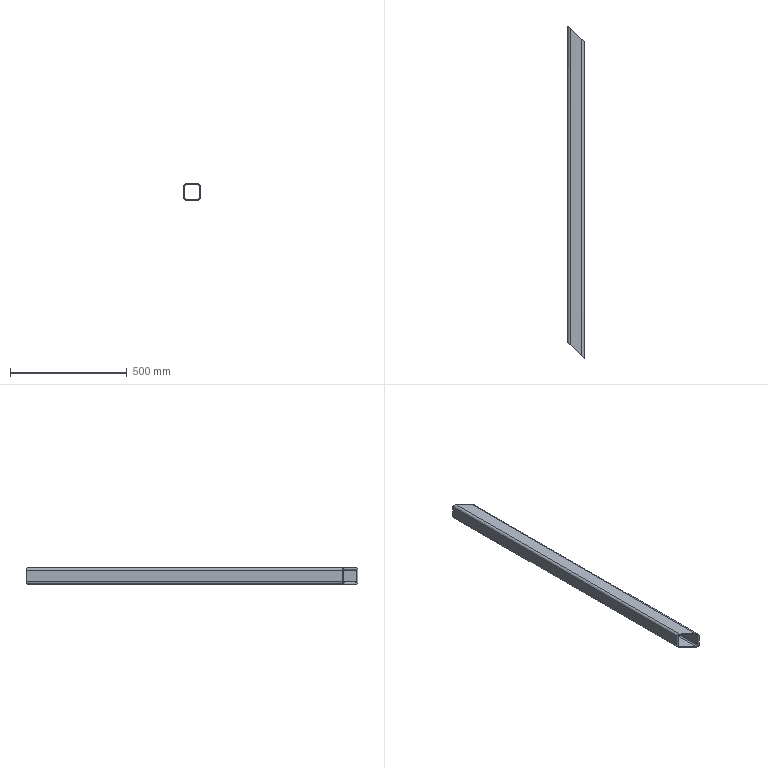Part | SolidWorks | features ICE 1, WeldMemberFeat 1, WeldmentFeature 1 | 1 solid | 18 faces | box 70 x 1421 x 70 mm | volume 1672765 mm3 | plane 10 | cylinder 8 | commonest cylinder face diameters 10 x4 20 x4
STEP:
#1=CARTESIAN_POINT('',(35.,1353.786,-25.));
#2=VERTEX_POINT('',#1);
#3=CARTESIAN_POINT('',(35.,0.,-25.));
#4=VERTEX_POINT('',#3);
#5=CARTESIAN_POINT('',(35.,1420.5,-25.));
#6=DIRECTION('',(0.,-1.,0.));
#7=VECTOR('',#6,1000.);
#8=LINE('',#5,#7);
#9=EDGE_CURVE('',#2,#4,#8,.T.);
#10=ORIENTED_EDGE('',*,*,#9,.F.);
#11=CARTESIAN_POINT('',(35.,1353.786,25.));
#12=VERTEX_POINT('',#11);
#13=CARTESIAN_POINT('',(35.,1353.786,-35.));
#14=DIRECTION('',(0.,0.,1.));
#15=VECTOR('',#14,1000.);
#16=LINE('',#13,#15);
#17=EDGE_CURVE('',#2,#12,#16,.T.);
#18=ORIENTED_EDGE('',*,*,#17,.T.);
#19=CARTESIAN_POINT('',(35.,0.,25.));
#20=VERTEX_POINT('',#19);
#21=CARTESIAN_POINT('',(35.,1420.5,25.));
#22=DIRECTION('',(0.,-1.,0.));
#23=VECTOR('',#22,1000.);
#24=LINE('',#21,#23);
#25=EDGE_CURVE('',#12,#20,#24,.T.);
#26=ORIENTED_EDGE('',*,*,#25,.T.);
#27=CARTESIAN_POINT('',(35.,0.,-25.));
#28=DIRECTION('',(0.,0.,-1.));
#29=VECTOR('',#28,1000.);
#30=LINE('',#27,#29);
#31=EDGE_CURVE('',#20,#4,#30,.T.);
#32=ORIENTED_EDGE('',*,*,#31,.T.);
#33=EDGE_LOOP('',(#10,#18,#26,#32));
#34=FACE_OUTER_BOUND('',#33,.T.);
#35=CARTESIAN_POINT('',(35.,1420.5,-25.));
#36=DIRECTION('',(-1.,0.,0.));
#37=DIRECTION('',(0.,0.,1.));
#38=AXIS2_PLACEMENT_3D('',#35,#36,#37);
#39=PLANE('',#38);
#40=ADVANCED_FACE('',(#34),#39,.F.);
#41=CARTESIAN_POINT('',(-35.,1420.5,-25.));
#42=VERTEX_POINT('',#41);
#43=CARTESIAN_POINT('',(-35.,66.714,-25.));
#44=VERTEX_POINT('',#43);
#45=CARTESIAN_POINT('',(-35.,1420.5,-25.));
#46=DIRECTION('',(0.,-1.,0.));
#47=VECTOR('',#46,1000.);
#48=LINE('',#45,#47);
#49=EDGE_CURVE('',#42,#44,#48,.T.);
#50=ORIENTED_EDGE('',*,*,#49,.T.);
#51=CARTESIAN_POINT('',(-35.,66.714,25.));
#52=VERTEX_POINT('',#51);
#53=CARTESIAN_POINT('',(-35.,66.714,-35.));
#54=DIRECTION('',(0.,0.,1.));
#55=VECTOR('',#54,1000.);
#56=LINE('',#53,#55);
#57=EDGE_CURVE('',#44,#52,#56,.T.);
#58=ORIENTED_EDGE('',*,*,#57,.T.);
#59=CARTESIAN_POINT('',(-35.,1420.5,25.));
#60=VERTEX_POINT('',#59);
#61=CARTESIAN_POINT('',(-35.,1420.5,25.));
#62=DIRECTION('',(0.,-1.,0.));
#63=VECTOR('',#62,1000.);
#64=LINE('',#61,#63);
#65=EDGE_CURVE('',#60,#52,#64,.T.);
#66=ORIENTED_EDGE('',*,*,#65,.F.);
#67=CARTESIAN_POINT('',(-35.,1420.5,25.));
#68=DIRECTION('',(0.,0.,1.));
#69=VECTOR('',#68,1000.);
#70=LINE('',#67,#69);
#71=EDGE_CURVE('',#42,#60,#70,.T.);
#72=ORIENTED_EDGE('',*,*,#71,.F.);
#73=EDGE_LOOP('',(#50,#58,#66,#72));
#74=FACE_OUTER_BOUND('',#73,.T.);
#75=CARTESIAN_POINT('',(-35.,1420.5,25.));
#76=DIRECTION('',(1.,0.,0.));
#77=DIRECTION('',(0.,0.,-1.));
#78=AXIS2_PLACEMENT_3D('',#75,#76,#77);
#79=PLANE('',#78);
#80=ADVANCED_FACE('',(#74),#79,.F.);
#81=ORIENTED_EDGE('',*,*,#49,.F.);
#82=CARTESIAN_POINT('',(-25.,1410.969,-35.));
#83=VERTEX_POINT('',#82);
#84=CARTESIAN_POINT('',(-35.,1420.5,-25.));
#85=CARTESIAN_POINT('',(-35.,1420.5,-30.858));
#86=CARTESIAN_POINT('',(-30.858,1416.552,-35.));
#87=CARTESIAN_POINT('',(-25.,1410.969,-35.));
#88=(BOUNDED_CURVE()B_SPLINE_CURVE(3,(#84,#85,#86,#87),.UNSPECIFIED.,.F.,.T.)B_SPLINE_CURVE_WITH_KNOTS((4,4),(3.142,4.712),.UNSPECIFIED.)CURVE()GEOMETRIC_REPRESENTATION_ITEM()RATIONAL_B_SPLINE_CURVE((1.,0.8047,0.8047,1.))REPRESENTATION_ITEM(''));
#89=EDGE_CURVE('',#42,#83,#88,.T.);
#90=ORIENTED_EDGE('',*,*,#89,.T.);
#91=CARTESIAN_POINT('',(-25.,57.183,-35.));
#92=VERTEX_POINT('',#91);
#93=CARTESIAN_POINT('',(-25.,1420.5,-35.));
#94=DIRECTION('',(0.,-1.,0.));
#95=VECTOR('',#94,1000.);
#96=LINE('',#93,#95);
#97=EDGE_CURVE('',#83,#92,#96,.T.);
#98=ORIENTED_EDGE('',*,*,#97,.T.);
#99=CARTESIAN_POINT('',(-25.,57.183,-35.));
#100=CARTESIAN_POINT('',(-30.858,62.766,-35.));
#101=CARTESIAN_POINT('',(-35.,66.714,-30.858));
#102=CARTESIAN_POINT('',(-35.,66.714,-25.));
#103=(BOUNDED_CURVE()B_SPLINE_CURVE(3,(#99,#100,#101,#102),.UNSPECIFIED.,.F.,.T.)B_SPLINE_CURVE_WITH_KNOTS((4,4),(1.571,3.142),.UNSPECIFIED.)CURVE()GEOMETRIC_REPRESENTATION_ITEM()RATIONAL_B_SPLINE_CURVE((1.,0.8047,0.8047,1.))REPRESENTATION_ITEM(''));
#104=EDGE_CURVE('',#92,#44,#103,.T.);
#105=ORIENTED_EDGE('',*,*,#104,.T.);
#106=EDGE_LOOP('',(#81,#90,#98,#105));
#107=FACE_OUTER_BOUND('',#106,.T.);
#108=CARTESIAN_POINT('',(-25.,1420.5,-25.));
#109=DIRECTION('',(0.,-1.,0.));
#110=DIRECTION('',(0.,0.,-1.));
#111=AXIS2_PLACEMENT_3D('',#108,#109,#110);
#112=CYLINDRICAL_SURFACE('',#111,10.);
#113=ADVANCED_FACE('',(#107),#112,.T.);
#114=ORIENTED_EDGE('',*,*,#97,.F.);
#115=CARTESIAN_POINT('',(25.,1363.317,-35.));
#116=VERTEX_POINT('',#115);
#117=CARTESIAN_POINT('',(-35.,1420.5,-35.));
#118=DIRECTION('',(0.7239,-0.6899,0.));
#119=VECTOR('',#118,1000.);
#120=LINE('',#117,#119);
#121=EDGE_CURVE('',#83,#116,#120,.T.);
#122=ORIENTED_EDGE('',*,*,#121,.T.);
#123=CARTESIAN_POINT('',(25.,9.531,-35.));
#124=VERTEX_POINT('',#123);
#125=CARTESIAN_POINT('',(25.,1420.5,-35.));
#126=DIRECTION('',(0.,-1.,0.));
#127=VECTOR('',#126,1000.);
#128=LINE('',#125,#127);
#129=EDGE_CURVE('',#116,#124,#128,.T.);
#130=ORIENTED_EDGE('',*,*,#129,.T.);
#131=CARTESIAN_POINT('',(-35.,66.714,-35.));
#132=DIRECTION('',(-0.7239,0.6899,0.));
#133=VECTOR('',#132,1000.);
#134=LINE('',#131,#133);
#135=EDGE_CURVE('',#124,#92,#134,.T.);
#136=ORIENTED_EDGE('',*,*,#135,.T.);
#137=EDGE_LOOP('',(#114,#122,#130,#136));
#138=FACE_OUTER_BOUND('',#137,.T.);
#139=CARTESIAN_POINT('',(25.,1420.5,-35.));
#140=DIRECTION('',(0.,0.,1.));
#141=DIRECTION('',(1.,0.,0.));
#142=AXIS2_PLACEMENT_3D('',#139,#140,#141);
#143=PLANE('',#142);
#144=ADVANCED_FACE('',(#138),#143,.F.);
#145=ORIENTED_EDGE('',*,*,#129,.F.);
#146=CARTESIAN_POINT('',(25.,1363.317,-35.));
#147=CARTESIAN_POINT('',(30.858,1357.734,-35.));
#148=CARTESIAN_POINT('',(35.,1353.786,-30.858));
#149=CARTESIAN_POINT('',(35.,1353.786,-25.));
#150=(BOUNDED_CURVE()B_SPLINE_CURVE(3,(#146,#147,#148,#149),.UNSPECIFIED.,.F.,.F.)B_SPLINE_CURVE_WITH_KNOTS((4,4),(4.712,6.283),.UNSPECIFIED.)CURVE()GEOMETRIC_REPRESENTATION_ITEM()RATIONAL_B_SPLINE_CURVE((1.,0.8047,0.8047,1.))REPRESENTATION_ITEM(''));
#151=EDGE_CURVE('',#116,#2,#150,.T.);
#152=ORIENTED_EDGE('',*,*,#151,.T.);
#153=ORIENTED_EDGE('',*,*,#9,.T.);
#154=CARTESIAN_POINT('',(35.,0.,-25.));
#155=CARTESIAN_POINT('',(35.,0.,-30.858));
#156=CARTESIAN_POINT('',(30.858,3.948,-35.));
#157=CARTESIAN_POINT('',(25.,9.531,-35.));
#158=(BOUNDED_CURVE()B_SPLINE_CURVE(3,(#154,#155,#156,#157),.UNSPECIFIED.,.F.,.F.)B_SPLINE_CURVE_WITH_KNOTS((4,4),(0.,1.571),.UNSPECIFIED.)CURVE()GEOMETRIC_REPRESENTATION_ITEM()RATIONAL_B_SPLINE_CURVE((1.,0.8047,0.8047,1.))REPRESENTATION_ITEM(''));
#159=EDGE_CURVE('',#4,#124,#158,.T.);
#160=ORIENTED_EDGE('',*,*,#159,.T.);
#161=EDGE_LOOP('',(#145,#152,#153,#160));
#162=FACE_OUTER_BOUND('',#161,.T.);
#163=CARTESIAN_POINT('',(25.,1420.5,-25.));
#164=DIRECTION('',(0.,-1.,0.));
#165=DIRECTION('',(0.,0.,-1.));
#166=AXIS2_PLACEMENT_3D('',#163,#164,#165);
#167=CYLINDRICAL_SURFACE('',#166,10.);
#168=ADVANCED_FACE('',(#162),#167,.T.);
#169=ORIENTED_EDGE('',*,*,#25,.F.);
#170=CARTESIAN_POINT('',(25.,1363.317,35.));
#171=VERTEX_POINT('',#170);
#172=CARTESIAN_POINT('',(35.,1353.786,25.));
#173=CARTESIAN_POINT('',(35.,1353.786,30.858));
#174=CARTESIAN_POINT('',(30.858,1357.734,35.));
#175=CARTESIAN_POINT('',(25.,1363.317,35.));
#176=(BOUNDED_CURVE()B_SPLINE_CURVE(3,(#172,#173,#174,#175),.UNSPECIFIED.,.F.,.F.)B_SPLINE_CURVE_WITH_KNOTS((4,4),(0.,1.571),.UNSPECIFIED.)CURVE()GEOMETRIC_REPRESENTATION_ITEM()RATIONAL_B_SPLINE_CURVE((1.,0.8047,0.8047,1.))REPRESENTATION_ITEM(''));
#177=EDGE_CURVE('',#12,#171,#176,.T.);
#178=ORIENTED_EDGE('',*,*,#177,.T.);
#179=CARTESIAN_POINT('',(25.,9.531,35.));
#180=VERTEX_POINT('',#179);
#181=CARTESIAN_POINT('',(25.,1420.5,35.));
#182=DIRECTION('',(0.,-1.,0.));
#183=VECTOR('',#182,1000.);
#184=LINE('',#181,#183);
#185=EDGE_CURVE('',#171,#180,#184,.T.);
#186=ORIENTED_EDGE('',*,*,#185,.T.);
#187=CARTESIAN_POINT('',(25.,9.531,35.));
#188=CARTESIAN_POINT('',(30.858,3.948,35.));
#189=CARTESIAN_POINT('',(35.,0.,30.858));
#190=CARTESIAN_POINT('',(35.,0.,25.));
#191=(BOUNDED_CURVE()B_SPLINE_CURVE(3,(#187,#188,#189,#190),.UNSPECIFIED.,.F.,.T.)B_SPLINE_CURVE_WITH_KNOTS((4,4),(4.712,6.283),.UNSPECIFIED.)CURVE()GEOMETRIC_REPRESENTATION_ITEM()RATIONAL_B_SPLINE_CURVE((1.,0.8047,0.8047,1.))REPRESENTATION_ITEM(''));
#192=EDGE_CURVE('',#180,#20,#191,.T.);
#193=ORIENTED_EDGE('',*,*,#192,.T.);
#194=EDGE_LOOP('',(#169,#178,#186,#193));
#195=FACE_OUTER_BOUND('',#194,.T.);
#196=CARTESIAN_POINT('',(25.,1420.5,25.));
#197=DIRECTION('',(0.,-1.,0.));
#198=DIRECTION('',(0.,0.,-1.));
#199=AXIS2_PLACEMENT_3D('',#196,#197,#198);
#200=CYLINDRICAL_SURFACE('',#199,10.);
#201=ADVANCED_FACE('',(#195),#200,.T.);
#202=ORIENTED_EDGE('',*,*,#185,.F.);
#203=CARTESIAN_POINT('',(-25.,1410.969,35.));
#204=VERTEX_POINT('',#203);
#205=CARTESIAN_POINT('',(-29.76,1415.506,35.));
#206=DIRECTION('',(-0.7239,0.6899,0.));
#207=VECTOR('',#206,1000.);
#208=LINE('',#205,#207);
#209=EDGE_CURVE('',#171,#204,#208,.T.);
#210=ORIENTED_EDGE('',*,*,#209,.T.);
#211=CARTESIAN_POINT('',(-25.,57.183,35.));
#212=VERTEX_POINT('',#211);
#213=CARTESIAN_POINT('',(-25.,1420.5,35.));
#214=DIRECTION('',(0.,-1.,0.));
#215=VECTOR('',#214,1000.);
#216=LINE('',#213,#215);
#217=EDGE_CURVE('',#204,#212,#216,.T.);
#218=ORIENTED_EDGE('',*,*,#217,.T.);
#219=CARTESIAN_POINT('',(-705.871,706.088,35.));
#220=DIRECTION('',(0.7239,-0.6899,0.));
#221=VECTOR('',#220,1000.);
#222=LINE('',#219,#221);
#223=EDGE_CURVE('',#212,#180,#222,.T.);
#224=ORIENTED_EDGE('',*,*,#223,.T.);
#225=EDGE_LOOP('',(#202,#210,#218,#224));
#226=FACE_OUTER_BOUND('',#225,.T.);
#227=CARTESIAN_POINT('',(-25.,1420.5,35.));
#228=DIRECTION('',(0.,0.,-1.));
#229=DIRECTION('',(-1.,0.,0.));
#230=AXIS2_PLACEMENT_3D('',#227,#228,#229);
#231=PLANE('',#230);
#232=ADVANCED_FACE('',(#226),#231,.F.);
#233=ORIENTED_EDGE('',*,*,#217,.F.);
#234=CARTESIAN_POINT('',(-25.,1410.969,35.));
#235=CARTESIAN_POINT('',(-30.858,1416.552,35.));
#236=CARTESIAN_POINT('',(-35.,1420.5,30.858));
#237=CARTESIAN_POINT('',(-35.,1420.5,25.));
#238=(BOUNDED_CURVE()B_SPLINE_CURVE(3,(#234,#235,#236,#237),.UNSPECIFIED.,.F.,.F.)B_SPLINE_CURVE_WITH_KNOTS((4,4),(1.571,3.142),.UNSPECIFIED.)CURVE()GEOMETRIC_REPRESENTATION_ITEM()RATIONAL_B_SPLINE_CURVE((1.,0.8047,0.8047,1.))REPRESENTATION_ITEM(''));
#239=EDGE_CURVE('',#204,#60,#238,.T.);
#240=ORIENTED_EDGE('',*,*,#239,.T.);
#241=ORIENTED_EDGE('',*,*,#65,.T.);
#242=CARTESIAN_POINT('',(-35.,66.714,25.));
#243=CARTESIAN_POINT('',(-35.,66.714,30.858));
#244=CARTESIAN_POINT('',(-30.858,62.766,35.));
#245=CARTESIAN_POINT('',(-25.,57.183,35.));
#246=(BOUNDED_CURVE()B_SPLINE_CURVE(3,(#242,#243,#244,#245),.UNSPECIFIED.,.F.,.F.)B_SPLINE_CURVE_WITH_KNOTS((4,4),(3.142,4.712),.UNSPECIFIED.)CURVE()GEOMETRIC_REPRESENTATION_ITEM()RATIONAL_B_SPLINE_CURVE((1.,0.8047,0.8047,1.))REPRESENTATION_ITEM(''));
#247=EDGE_CURVE('',#52,#212,#246,.T.);
#248=ORIENTED_EDGE('',*,*,#247,.T.);
#249=EDGE_LOOP('',(#233,#240,#241,#248));
#250=FACE_OUTER_BOUND('',#249,.T.);
#251=CARTESIAN_POINT('',(-25.,1420.5,25.));
#252=DIRECTION('',(0.,-1.,0.));
#253=DIRECTION('',(0.,0.,-1.));
#254=AXIS2_PLACEMENT_3D('',#251,#252,#253);
#255=CYLINDRICAL_SURFACE('',#254,10.);
#256=ADVANCED_FACE('',(#250),#255,.T.);
#257=CARTESIAN_POINT('',(25.,9.531,30.));
#258=VERTEX_POINT('',#257);
#259=CARTESIAN_POINT('',(30.,4.765,25.));
#260=VERTEX_POINT('',#259);
#261=CARTESIAN_POINT('',(25.,9.531,30.));
#262=CARTESIAN_POINT('',(27.929,6.739,30.));
#263=CARTESIAN_POINT('',(30.,4.765,27.929));
#264=CARTESIAN_POINT('',(30.,4.765,25.));
#265=(BOUNDED_CURVE()B_SPLINE_CURVE(3,(#261,#262,#263,#264),.UNSPECIFIED.,.F.,.F.)B_SPLINE_CURVE_WITH_KNOTS((4,4),(4.712,6.283),.UNSPECIFIED.)CURVE()GEOMETRIC_REPRESENTATION_ITEM()RATIONAL_B_SPLINE_CURVE((1.,0.8047,0.8047,1.))REPRESENTATION_ITEM(''));
#266=EDGE_CURVE('',#258,#260,#265,.T.);
#267=ORIENTED_EDGE('',*,*,#266,.T.);
#268=CARTESIAN_POINT('',(30.,4.765,-25.));
#269=VERTEX_POINT('',#268);
#270=CARTESIAN_POINT('',(30.,4.765,-25.));
#271=DIRECTION('',(0.,0.,-1.));
#272=VECTOR('',#271,1000.);
#273=LINE('',#270,#272);
#274=EDGE_CURVE('',#260,#269,#273,.T.);
#275=ORIENTED_EDGE('',*,*,#274,.T.);
#276=CARTESIAN_POINT('',(25.,9.531,-30.));
#277=VERTEX_POINT('',#276);
#278=CARTESIAN_POINT('',(30.,4.765,-25.));
#279=CARTESIAN_POINT('',(30.,4.765,-27.929));
#280=CARTESIAN_POINT('',(27.929,6.739,-30.));
#281=CARTESIAN_POINT('',(25.,9.531,-30.));
#282=(BOUNDED_CURVE()B_SPLINE_CURVE(3,(#278,#279,#280,#281),.UNSPECIFIED.,.F.,.F.)B_SPLINE_CURVE_WITH_KNOTS((4,4),(0.,1.571),.UNSPECIFIED.)CURVE()GEOMETRIC_REPRESENTATION_ITEM()RATIONAL_B_SPLINE_CURVE((1.,0.8047,0.8047,1.))REPRESENTATION_ITEM(''));
#283=EDGE_CURVE('',#269,#277,#282,.T.);
#284=ORIENTED_EDGE('',*,*,#283,.T.);
#285=CARTESIAN_POINT('',(-25.,57.183,-30.));
#286=VERTEX_POINT('',#285);
#287=CARTESIAN_POINT('',(-679.67,681.117,-30.));
#288=DIRECTION('',(-0.7239,0.6899,0.));
#289=VECTOR('',#288,1000.);
#290=LINE('',#287,#289);
#291=EDGE_CURVE('',#277,#286,#290,.T.);
#292=ORIENTED_EDGE('',*,*,#291,.T.);
#293=CARTESIAN_POINT('',(-30.,61.948,-25.));
#294=VERTEX_POINT('',#293);
#295=CARTESIAN_POINT('',(-25.,57.183,-30.));
#296=CARTESIAN_POINT('',(-27.929,59.974,-30.));
#297=CARTESIAN_POINT('',(-30.,61.948,-27.929));
#298=CARTESIAN_POINT('',(-30.,61.948,-25.));
#299=(BOUNDED_CURVE()B_SPLINE_CURVE(3,(#295,#296,#297,#298),.UNSPECIFIED.,.F.,.F.)B_SPLINE_CURVE_WITH_KNOTS((4,4),(1.571,3.142),.UNSPECIFIED.)CURVE()GEOMETRIC_REPRESENTATION_ITEM()RATIONAL_B_SPLINE_CURVE((1.,0.8047,0.8047,1.))REPRESENTATION_ITEM(''));
#300=EDGE_CURVE('',#286,#294,#299,.T.);
#301=ORIENTED_EDGE('',*,*,#300,.T.);
#302=CARTESIAN_POINT('',(-30.,61.948,25.));
#303=VERTEX_POINT('',#302);
#304=CARTESIAN_POINT('',(-30.,61.948,25.));
#305=DIRECTION('',(0.,0.,1.));
#306=VECTOR('',#305,1000.);
#307=LINE('',#304,#306);
#308=EDGE_CURVE('',#294,#303,#307,.T.);
#309=ORIENTED_EDGE('',*,*,#308,.T.);
#310=CARTESIAN_POINT('',(-25.,57.183,30.));
#311=VERTEX_POINT('',#310);
#312=CARTESIAN_POINT('',(-30.,61.948,25.));
#313=CARTESIAN_POINT('',(-30.,61.948,27.929));
#314=CARTESIAN_POINT('',(-27.929,59.974,30.));
#315=CARTESIAN_POINT('',(-25.,57.183,30.));
#316=(BOUNDED_CURVE()B_SPLINE_CURVE(3,(#312,#313,#314,#315),.UNSPECIFIED.,.F.,.T.)B_SPLINE_CURVE_WITH_KNOTS((4,4),(3.142,4.712),.UNSPECIFIED.)CURVE()GEOMETRIC_REPRESENTATION_ITEM()RATIONAL_B_SPLINE_CURVE((1.,0.8047,0.8047,1.))REPRESENTATION_ITEM(''));
#317=EDGE_CURVE('',#303,#311,#316,.T.);
#318=ORIENTED_EDGE('',*,*,#317,.T.);
#319=CARTESIAN_POINT('',(-705.871,706.088,30.));
#320=DIRECTION('',(0.7239,-0.6899,0.));
#321=VECTOR('',#320,1000.);
#322=LINE('',#319,#321);
#323=EDGE_CURVE('',#311,#258,#322,.T.);
#324=ORIENTED_EDGE('',*,*,#323,.T.);
#325=EDGE_LOOP('',(#267,#275,#284,#292,#301,#309,#318,#324));
#326=FACE_BOUND('',#325,.T.);
#327=ORIENTED_EDGE('',*,*,#57,.F.);
#328=ORIENTED_EDGE('',*,*,#104,.F.);
#329=ORIENTED_EDGE('',*,*,#135,.F.);
#330=ORIENTED_EDGE('',*,*,#159,.F.);
#331=ORIENTED_EDGE('',*,*,#31,.F.);
#332=ORIENTED_EDGE('',*,*,#192,.F.);
#333=ORIENTED_EDGE('',*,*,#223,.F.);
#334=ORIENTED_EDGE('',*,*,#247,.F.);
#335=EDGE_LOOP('',(#327,#328,#329,#330,#331,#332,#333,#334));
#336=FACE_OUTER_BOUND('',#335,.T.);
#337=CARTESIAN_POINT('',(-35.,66.714,-35.));
#338=DIRECTION('',(0.6899,0.7239,0.));
#339=DIRECTION('',(-0.7239,0.6899,0.));
#340=AXIS2_PLACEMENT_3D('',#337,#338,#339);
#341=PLANE('',#340);
#342=ADVANCED_FACE('',(#326,#336),#341,.F.);
#343=CARTESIAN_POINT('',(30.,1358.552,25.));
#344=VERTEX_POINT('',#343);
#345=CARTESIAN_POINT('',(25.,1363.317,30.));
#346=VERTEX_POINT('',#345);
#347=CARTESIAN_POINT('',(30.,1358.552,25.));
#348=CARTESIAN_POINT('',(30.,1358.552,27.929));
#349=CARTESIAN_POINT('',(27.929,1360.526,30.));
#350=CARTESIAN_POINT('',(25.,1363.317,30.));
#351=(BOUNDED_CURVE()B_SPLINE_CURVE(3,(#347,#348,#349,#350),.UNSPECIFIED.,.F.,.F.)B_SPLINE_CURVE_WITH_KNOTS((4,4),(0.,1.571),.UNSPECIFIED.)CURVE()GEOMETRIC_REPRESENTATION_ITEM()RATIONAL_B_SPLINE_CURVE((1.,0.8047,0.8047,1.))REPRESENTATION_ITEM(''));
#352=EDGE_CURVE('',#344,#346,#351,.T.);
#353=ORIENTED_EDGE('',*,*,#352,.T.);
#354=CARTESIAN_POINT('',(-25.,1410.969,30.));
#355=VERTEX_POINT('',#354);
#356=CARTESIAN_POINT('',(-29.76,1415.506,30.));
#357=DIRECTION('',(-0.7239,0.6899,0.));
#358=VECTOR('',#357,1000.);
#359=LINE('',#356,#358);
#360=EDGE_CURVE('',#346,#355,#359,.T.);
#361=ORIENTED_EDGE('',*,*,#360,.T.);
#362=CARTESIAN_POINT('',(-30.,1415.735,25.));
#363=VERTEX_POINT('',#362);
#364=CARTESIAN_POINT('',(-25.,1410.969,30.));
#365=CARTESIAN_POINT('',(-27.929,1413.761,30.));
#366=CARTESIAN_POINT('',(-30.,1415.735,27.929));
#367=CARTESIAN_POINT('',(-30.,1415.735,25.));
#368=(BOUNDED_CURVE()B_SPLINE_CURVE(3,(#364,#365,#366,#367),.UNSPECIFIED.,.F.,.F.)B_SPLINE_CURVE_WITH_KNOTS((4,4),(1.571,3.142),.UNSPECIFIED.)CURVE()GEOMETRIC_REPRESENTATION_ITEM()RATIONAL_B_SPLINE_CURVE((1.,0.8047,0.8047,1.))REPRESENTATION_ITEM(''));
#369=EDGE_CURVE('',#355,#363,#368,.T.);
#370=ORIENTED_EDGE('',*,*,#369,.T.);
#371=CARTESIAN_POINT('',(-30.,1415.735,-25.));
#372=VERTEX_POINT('',#371);
#373=CARTESIAN_POINT('',(-30.,1415.735,25.));
#374=DIRECTION('',(0.,0.,-1.));
#375=VECTOR('',#374,1000.);
#376=LINE('',#373,#375);
#377=EDGE_CURVE('',#363,#372,#376,.T.);
#378=ORIENTED_EDGE('',*,*,#377,.T.);
#379=CARTESIAN_POINT('',(-25.,1410.969,-30.));
#380=VERTEX_POINT('',#379);
#381=CARTESIAN_POINT('',(-30.,1415.735,-25.));
#382=CARTESIAN_POINT('',(-30.,1415.735,-27.929));
#383=CARTESIAN_POINT('',(-27.929,1413.761,-30.));
#384=CARTESIAN_POINT('',(-25.,1410.969,-30.));
#385=(BOUNDED_CURVE()B_SPLINE_CURVE(3,(#381,#382,#383,#384),.UNSPECIFIED.,.F.,.F.)B_SPLINE_CURVE_WITH_KNOTS((4,4),(3.142,4.712),.UNSPECIFIED.)CURVE()GEOMETRIC_REPRESENTATION_ITEM()RATIONAL_B_SPLINE_CURVE((1.,0.8047,0.8047,1.))REPRESENTATION_ITEM(''));
#386=EDGE_CURVE('',#372,#380,#385,.T.);
#387=ORIENTED_EDGE('',*,*,#386,.T.);
#388=CARTESIAN_POINT('',(25.,1363.317,-30.));
#389=VERTEX_POINT('',#388);
#390=CARTESIAN_POINT('',(-3.559,1390.535,-30.));
#391=DIRECTION('',(0.7239,-0.6899,0.));
#392=VECTOR('',#391,1000.);
#393=LINE('',#390,#392);
#394=EDGE_CURVE('',#380,#389,#393,.T.);
#395=ORIENTED_EDGE('',*,*,#394,.T.);
#396=CARTESIAN_POINT('',(30.,1358.552,-25.));
#397=VERTEX_POINT('',#396);
#398=CARTESIAN_POINT('',(25.,1363.317,-30.));
#399=CARTESIAN_POINT('',(27.929,1360.526,-30.));
#400=CARTESIAN_POINT('',(30.,1358.552,-27.929));
#401=CARTESIAN_POINT('',(30.,1358.552,-25.));
#402=(BOUNDED_CURVE()B_SPLINE_CURVE(3,(#398,#399,#400,#401),.UNSPECIFIED.,.F.,.F.)B_SPLINE_CURVE_WITH_KNOTS((4,4),(4.712,6.283),.UNSPECIFIED.)CURVE()GEOMETRIC_REPRESENTATION_ITEM()RATIONAL_B_SPLINE_CURVE((1.,0.8047,0.8047,1.))REPRESENTATION_ITEM(''));
#403=EDGE_CURVE('',#389,#397,#402,.T.);
#404=ORIENTED_EDGE('',*,*,#403,.T.);
#405=CARTESIAN_POINT('',(30.,1358.552,-25.));
#406=DIRECTION('',(0.,0.,1.));
#407=VECTOR('',#406,1000.);
#408=LINE('',#405,#407);
#409=EDGE_CURVE('',#397,#344,#408,.T.);
#410=ORIENTED_EDGE('',*,*,#409,.T.);
#411=EDGE_LOOP('',(#353,#361,#370,#378,#387,#395,#404,#410));
#412=FACE_BOUND('',#411,.T.);
#413=ORIENTED_EDGE('',*,*,#209,.F.);
#414=ORIENTED_EDGE('',*,*,#177,.F.);
#415=ORIENTED_EDGE('',*,*,#17,.F.);
#416=ORIENTED_EDGE('',*,*,#151,.F.);
#417=ORIENTED_EDGE('',*,*,#121,.F.);
#418=ORIENTED_EDGE('',*,*,#89,.F.);
#419=ORIENTED_EDGE('',*,*,#71,.T.);
#420=ORIENTED_EDGE('',*,*,#239,.F.);
#421=EDGE_LOOP('',(#413,#414,#415,#416,#417,#418,#419,#420));
#422=FACE_OUTER_BOUND('',#421,.T.);
#423=CARTESIAN_POINT('',(-35.,1420.5,-35.));
#424=DIRECTION('',(-0.6899,-0.7239,0.));
#425=DIRECTION('',(0.7239,-0.6899,0.));
#426=AXIS2_PLACEMENT_3D('',#423,#424,#425);
#427=PLANE('',#426);
#428=ADVANCED_FACE('',(#412,#422),#427,.F.);
#429=ORIENTED_EDGE('',*,*,#352,.F.);
#430=CARTESIAN_POINT('',(30.,1420.5,25.));
#431=DIRECTION('',(0.,-1.,0.));
#432=VECTOR('',#431,1000.);
#433=LINE('',#430,#432);
#434=EDGE_CURVE('',#344,#260,#433,.T.);
#435=ORIENTED_EDGE('',*,*,#434,.T.);
#436=ORIENTED_EDGE('',*,*,#266,.F.);
#437=CARTESIAN_POINT('',(25.,1420.5,30.));
#438=DIRECTION('',(0.,-1.,0.));
#439=VECTOR('',#438,1000.);
#440=LINE('',#437,#439);
#441=EDGE_CURVE('',#346,#258,#440,.T.);
#442=ORIENTED_EDGE('',*,*,#441,.F.);
#443=EDGE_LOOP('',(#429,#435,#436,#442));
#444=FACE_OUTER_BOUND('',#443,.T.);
#445=CARTESIAN_POINT('',(25.,1420.5,25.));
#446=DIRECTION('',(0.,-1.,0.));
#447=DIRECTION('',(0.,0.,-1.));
#448=AXIS2_PLACEMENT_3D('',#445,#446,#447);
#449=CYLINDRICAL_SURFACE('',#448,5.);
#450=ADVANCED_FACE('',(#444),#449,.F.);
#451=ORIENTED_EDGE('',*,*,#360,.F.);
#452=ORIENTED_EDGE('',*,*,#441,.T.);
#453=ORIENTED_EDGE('',*,*,#323,.F.);
#454=CARTESIAN_POINT('',(-25.,1420.5,30.));
#455=DIRECTION('',(0.,-1.,0.));
#456=VECTOR('',#455,1000.);
#457=LINE('',#454,#456);
#458=EDGE_CURVE('',#355,#311,#457,.T.);
#459=ORIENTED_EDGE('',*,*,#458,.F.);
#460=EDGE_LOOP('',(#451,#452,#453,#459));
#461=FACE_OUTER_BOUND('',#460,.T.);
#462=CARTESIAN_POINT('',(-25.,1420.5,30.));
#463=DIRECTION('',(0.,0.,-1.));
#464=DIRECTION('',(-1.,0.,0.));
#465=AXIS2_PLACEMENT_3D('',#462,#463,#464);
#466=PLANE('',#465);
#467=ADVANCED_FACE('',(#461),#466,.T.);
#468=ORIENTED_EDGE('',*,*,#369,.F.);
#469=ORIENTED_EDGE('',*,*,#458,.T.);
#470=ORIENTED_EDGE('',*,*,#317,.F.);
#471=CARTESIAN_POINT('',(-30.,1420.5,25.));
#472=DIRECTION('',(0.,-1.,0.));
#473=VECTOR('',#472,1000.);
#474=LINE('',#471,#473);
#475=EDGE_CURVE('',#363,#303,#474,.T.);
#476=ORIENTED_EDGE('',*,*,#475,.F.);
#477=EDGE_LOOP('',(#468,#469,#470,#476));
#478=FACE_OUTER_BOUND('',#477,.T.);
#479=CARTESIAN_POINT('',(-25.,1420.5,25.));
#480=DIRECTION('',(0.,-1.,0.));
#481=DIRECTION('',(0.,0.,-1.));
#482=AXIS2_PLACEMENT_3D('',#479,#480,#481);
#483=CYLINDRICAL_SURFACE('',#482,5.);
#484=ADVANCED_FACE('',(#478),#483,.F.);
#485=ORIENTED_EDGE('',*,*,#377,.F.);
#486=ORIENTED_EDGE('',*,*,#475,.T.);
#487=ORIENTED_EDGE('',*,*,#308,.F.);
#488=CARTESIAN_POINT('',(-30.,1420.5,-25.));
#489=DIRECTION('',(0.,-1.,0.));
#490=VECTOR('',#489,1000.);
#491=LINE('',#488,#490);
#492=EDGE_CURVE('',#372,#294,#491,.T.);
#493=ORIENTED_EDGE('',*,*,#492,.F.);
#494=EDGE_LOOP('',(#485,#486,#487,#493));
#495=FACE_OUTER_BOUND('',#494,.T.);
#496=CARTESIAN_POINT('',(-30.,1420.5,25.));
#497=DIRECTION('',(1.,0.,0.));
#498=DIRECTION('',(0.,0.,-1.));
#499=AXIS2_PLACEMENT_3D('',#496,#497,#498);
#500=PLANE('',#499);
#501=ADVANCED_FACE('',(#495),#500,.T.);
#502=ORIENTED_EDGE('',*,*,#386,.F.);
#503=ORIENTED_EDGE('',*,*,#492,.T.);
#504=ORIENTED_EDGE('',*,*,#300,.F.);
#505=CARTESIAN_POINT('',(-25.,1420.5,-30.));
#506=DIRECTION('',(0.,-1.,0.));
#507=VECTOR('',#506,1000.);
#508=LINE('',#505,#507);
#509=EDGE_CURVE('',#380,#286,#508,.T.);
#510=ORIENTED_EDGE('',*,*,#509,.F.);
#511=EDGE_LOOP('',(#502,#503,#504,#510));
#512=FACE_OUTER_BOUND('',#511,.T.);
#513=CARTESIAN_POINT('',(-25.,1420.5,-25.));
#514=DIRECTION('',(0.,-1.,0.));
#515=DIRECTION('',(0.,0.,-1.));
#516=AXIS2_PLACEMENT_3D('',#513,#514,#515);
#517=CYLINDRICAL_SURFACE('',#516,5.);
#518=ADVANCED_FACE('',(#512),#517,.F.);
#519=ORIENTED_EDGE('',*,*,#394,.F.);
#520=ORIENTED_EDGE('',*,*,#509,.T.);
#521=ORIENTED_EDGE('',*,*,#291,.F.);
#522=CARTESIAN_POINT('',(25.,1420.5,-30.));
#523=DIRECTION('',(0.,-1.,0.));
#524=VECTOR('',#523,1000.);
#525=LINE('',#522,#524);
#526=EDGE_CURVE('',#389,#277,#525,.T.);
#527=ORIENTED_EDGE('',*,*,#526,.F.);
#528=EDGE_LOOP('',(#519,#520,#521,#527));
#529=FACE_OUTER_BOUND('',#528,.T.);
#530=CARTESIAN_POINT('',(25.,1420.5,-30.));
#531=DIRECTION('',(0.,0.,1.));
#532=DIRECTION('',(1.,0.,0.));
#533=AXIS2_PLACEMENT_3D('',#530,#531,#532);
#534=PLANE('',#533);
#535=ADVANCED_FACE('',(#529),#534,.T.);
#536=ORIENTED_EDGE('',*,*,#403,.F.);
#537=ORIENTED_EDGE('',*,*,#526,.T.);
#538=ORIENTED_EDGE('',*,*,#283,.F.);
#539=CARTESIAN_POINT('',(30.,1420.5,-25.));
#540=DIRECTION('',(0.,-1.,0.));
#541=VECTOR('',#540,1000.);
#542=LINE('',#539,#541);
#543=EDGE_CURVE('',#397,#269,#542,.T.);
#544=ORIENTED_EDGE('',*,*,#543,.F.);
#545=EDGE_LOOP('',(#536,#537,#538,#544));
#546=FACE_OUTER_BOUND('',#545,.T.);
#547=CARTESIAN_POINT('',(25.,1420.5,-25.));
#548=DIRECTION('',(0.,-1.,0.));
#549=DIRECTION('',(0.,0.,-1.));
#550=AXIS2_PLACEMENT_3D('',#547,#548,#549);
#551=CYLINDRICAL_SURFACE('',#550,5.);
#552=ADVANCED_FACE('',(#546),#551,.F.);
#553=ORIENTED_EDGE('',*,*,#409,.F.);
#554=ORIENTED_EDGE('',*,*,#543,.T.);
#555=ORIENTED_EDGE('',*,*,#274,.F.);
#556=ORIENTED_EDGE('',*,*,#434,.F.);
#557=EDGE_LOOP('',(#553,#554,#555,#556));
#558=FACE_OUTER_BOUND('',#557,.T.);
#559=CARTESIAN_POINT('',(30.,1420.5,-25.));
#560=DIRECTION('',(-1.,0.,0.));
#561=DIRECTION('',(0.,0.,1.));
#562=AXIS2_PLACEMENT_3D('',#559,#560,#561);
#563=PLANE('',#562);
#564=ADVANCED_FACE('',(#558),#563,.T.);
#565=CLOSED_SHELL('',(#40,#80,#113,#144,#168,#201,#232,#256,#342,#428,#450,#467,#484,#501,#518,#535,#552,#564));
#566=MANIFOLD_SOLID_BREP('',#565);
#567=CARTESIAN_POINT('',(0.,0.,0.));
#568=DIRECTION('',(0.,0.,1.));
#569=DIRECTION('',(1.,0.,0.));
#570=AXIS2_PLACEMENT_3D('',#567,#568,#569);
#571=(LENGTH_UNIT()NAMED_UNIT(*)SI_UNIT(.MILLI.,.METRE.));
#572=UNCERTAINTY_MEASURE_WITH_UNIT(LENGTH_MEASURE(0.00001),#571,'','');
#573=(NAMED_UNIT(*)PLANE_ANGLE_UNIT()SI_UNIT($,.RADIAN.));
#574=(NAMED_UNIT(*)SI_UNIT($,.STERADIAN.)SOLID_ANGLE_UNIT());
#575=(GEOMETRIC_REPRESENTATION_CONTEXT(3)GLOBAL_UNCERTAINTY_ASSIGNED_CONTEXT((#572))GLOBAL_UNIT_ASSIGNED_CONTEXT((#571,#573,#574))REPRESENTATION_CONTEXT('',''));
#576=ADVANCED_BREP_SHAPE_REPRESENTATION('',(#566,#570),#575);